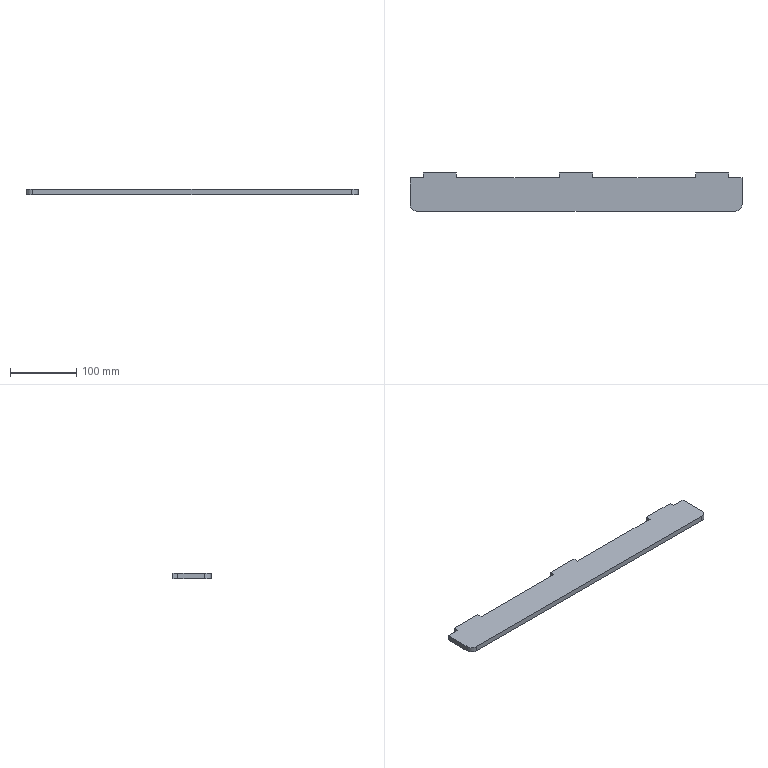Part | SolidWorks | features FlatPattern 1, SMBaseFlange 1, SheetMetal 1 | 1 solid | 20 faces | box 500 x 57.5 x 8 mm | volume 208657 mm3 | plane 18 | cylinder 2 | commonest cylinder face diameters 20 x2
STEP:
#1=CARTESIAN_POINT('',(-172.817,-291.5,0.));
#2=VERTEX_POINT('',#1);
#3=CARTESIAN_POINT('',(-192.817,-291.5,0.));
#4=VERTEX_POINT('',#3);
#5=CARTESIAN_POINT('',(-172.817,-291.5,0.));
#6=DIRECTION('',(-1.,0.,0.));
#7=VECTOR('',#6,1000.);
#8=LINE('',#5,#7);
#9=EDGE_CURVE('',#2,#4,#8,.T.);
#10=ORIENTED_EDGE('',*,*,#9,.F.);
#11=CARTESIAN_POINT('',(-172.817,-291.5,-8.));
#12=VERTEX_POINT('',#11);
#13=CARTESIAN_POINT('',(-172.817,-291.5,-8.));
#14=DIRECTION('',(0.,0.,1.));
#15=VECTOR('',#14,1000.);
#16=LINE('',#13,#15);
#17=EDGE_CURVE('',#12,#2,#16,.T.);
#18=ORIENTED_EDGE('',*,*,#17,.F.);
#19=CARTESIAN_POINT('',(-192.817,-291.5,-8.));
#20=VERTEX_POINT('',#19);
#21=CARTESIAN_POINT('',(-172.817,-291.5,-8.));
#22=DIRECTION('',(-1.,0.,0.));
#23=VECTOR('',#22,1000.);
#24=LINE('',#21,#23);
#25=EDGE_CURVE('',#12,#20,#24,.T.);
#26=ORIENTED_EDGE('',*,*,#25,.T.);
#27=CARTESIAN_POINT('',(-192.817,-291.5,-8.));
#28=DIRECTION('',(0.,0.,1.));
#29=VECTOR('',#28,1000.);
#30=LINE('',#27,#29);
#31=EDGE_CURVE('',#20,#4,#30,.T.);
#32=ORIENTED_EDGE('',*,*,#31,.T.);
#33=EDGE_LOOP('',(#10,#18,#26,#32));
#34=FACE_OUTER_BOUND('',#33,.T.);
#35=CARTESIAN_POINT('',(-172.817,-291.5,-8.));
#36=DIRECTION('',(0.,1.,0.));
#37=DIRECTION('',(0.,0.,1.));
#38=AXIS2_PLACEMENT_3D('',#35,#36,#37);
#39=PLANE('',#38);
#40=ADVANCED_FACE('',(#34),#39,.T.);
#41=CARTESIAN_POINT('',(-172.817,-284.,0.));
#42=VERTEX_POINT('',#41);
#43=CARTESIAN_POINT('',(-172.817,-284.,0.));
#44=DIRECTION('',(0.,-1.,0.));
#45=VECTOR('',#44,1000.);
#46=LINE('',#43,#45);
#47=EDGE_CURVE('',#42,#2,#46,.T.);
#48=ORIENTED_EDGE('',*,*,#47,.F.);
#49=CARTESIAN_POINT('',(-172.817,-284.,-8.));
#50=VERTEX_POINT('',#49);
#51=CARTESIAN_POINT('',(-172.817,-284.,-8.));
#52=DIRECTION('',(0.,0.,1.));
#53=VECTOR('',#52,1000.);
#54=LINE('',#51,#53);
#55=EDGE_CURVE('',#50,#42,#54,.T.);
#56=ORIENTED_EDGE('',*,*,#55,.F.);
#57=CARTESIAN_POINT('',(-172.817,-284.,-8.));
#58=DIRECTION('',(0.,-1.,0.));
#59=VECTOR('',#58,1000.);
#60=LINE('',#57,#59);
#61=EDGE_CURVE('',#50,#12,#60,.T.);
#62=ORIENTED_EDGE('',*,*,#61,.T.);
#63=ORIENTED_EDGE('',*,*,#17,.T.);
#64=EDGE_LOOP('',(#48,#56,#62,#63));
#65=FACE_OUTER_BOUND('',#64,.T.);
#66=CARTESIAN_POINT('',(-172.817,-284.,-8.));
#67=DIRECTION('',(-1.,0.,0.));
#68=DIRECTION('',(0.,-1.,0.));
#69=AXIS2_PLACEMENT_3D('',#66,#67,#68);
#70=PLANE('',#69);
#71=ADVANCED_FACE('',(#65),#70,.T.);
#72=CARTESIAN_POINT('',(-122.817,-284.,0.));
#73=VERTEX_POINT('',#72);
#74=CARTESIAN_POINT('',(-122.817,-284.,0.));
#75=DIRECTION('',(-1.,0.,0.));
#76=VECTOR('',#75,1000.);
#77=LINE('',#74,#76);
#78=EDGE_CURVE('',#73,#42,#77,.T.);
#79=ORIENTED_EDGE('',*,*,#78,.F.);
#80=CARTESIAN_POINT('',(-122.817,-284.,-8.));
#81=VERTEX_POINT('',#80);
#82=CARTESIAN_POINT('',(-122.817,-284.,-8.));
#83=DIRECTION('',(0.,0.,1.));
#84=VECTOR('',#83,1000.);
#85=LINE('',#82,#84);
#86=EDGE_CURVE('',#81,#73,#85,.T.);
#87=ORIENTED_EDGE('',*,*,#86,.F.);
#88=CARTESIAN_POINT('',(-122.817,-284.,-8.));
#89=DIRECTION('',(-1.,0.,0.));
#90=VECTOR('',#89,1000.);
#91=LINE('',#88,#90);
#92=EDGE_CURVE('',#81,#50,#91,.T.);
#93=ORIENTED_EDGE('',*,*,#92,.T.);
#94=ORIENTED_EDGE('',*,*,#55,.T.);
#95=EDGE_LOOP('',(#79,#87,#93,#94));
#96=FACE_OUTER_BOUND('',#95,.T.);
#97=CARTESIAN_POINT('',(-122.817,-284.,-8.));
#98=DIRECTION('',(0.,1.,0.));
#99=DIRECTION('',(0.,0.,1.));
#100=AXIS2_PLACEMENT_3D('',#97,#98,#99);
#101=PLANE('',#100);
#102=ADVANCED_FACE('',(#96),#101,.T.);
#103=CARTESIAN_POINT('',(-122.817,-291.5,0.));
#104=VERTEX_POINT('',#103);
#105=CARTESIAN_POINT('',(-122.817,-291.5,0.));
#106=DIRECTION('',(0.,1.,0.));
#107=VECTOR('',#106,1000.);
#108=LINE('',#105,#107);
#109=EDGE_CURVE('',#104,#73,#108,.T.);
#110=ORIENTED_EDGE('',*,*,#109,.F.);
#111=CARTESIAN_POINT('',(-122.817,-291.5,-8.));
#112=VERTEX_POINT('',#111);
#113=CARTESIAN_POINT('',(-122.817,-291.5,-8.));
#114=DIRECTION('',(0.,0.,1.));
#115=VECTOR('',#114,1000.);
#116=LINE('',#113,#115);
#117=EDGE_CURVE('',#112,#104,#116,.T.);
#118=ORIENTED_EDGE('',*,*,#117,.F.);
#119=CARTESIAN_POINT('',(-122.817,-291.5,-8.));
#120=DIRECTION('',(0.,1.,0.));
#121=VECTOR('',#120,1000.);
#122=LINE('',#119,#121);
#123=EDGE_CURVE('',#112,#81,#122,.T.);
#124=ORIENTED_EDGE('',*,*,#123,.T.);
#125=ORIENTED_EDGE('',*,*,#86,.T.);
#126=EDGE_LOOP('',(#110,#118,#124,#125));
#127=FACE_OUTER_BOUND('',#126,.T.);
#128=CARTESIAN_POINT('',(-122.817,-291.5,-8.));
#129=DIRECTION('',(1.,0.,0.));
#130=DIRECTION('',(0.,0.,-1.));
#131=AXIS2_PLACEMENT_3D('',#128,#129,#130);
#132=PLANE('',#131);
#133=ADVANCED_FACE('',(#127),#132,.T.);
#134=CARTESIAN_POINT('',(32.183,-291.5,0.));
#135=VERTEX_POINT('',#134);
#136=CARTESIAN_POINT('',(32.183,-291.5,0.));
#137=DIRECTION('',(-1.,0.,0.));
#138=VECTOR('',#137,1000.);
#139=LINE('',#136,#138);
#140=EDGE_CURVE('',#135,#104,#139,.T.);
#141=ORIENTED_EDGE('',*,*,#140,.F.);
#142=CARTESIAN_POINT('',(32.183,-291.5,-8.));
#143=VERTEX_POINT('',#142);
#144=CARTESIAN_POINT('',(32.183,-291.5,-8.));
#145=DIRECTION('',(0.,0.,1.));
#146=VECTOR('',#145,1000.);
#147=LINE('',#144,#146);
#148=EDGE_CURVE('',#143,#135,#147,.T.);
#149=ORIENTED_EDGE('',*,*,#148,.F.);
#150=CARTESIAN_POINT('',(32.183,-291.5,-8.));
#151=DIRECTION('',(-1.,0.,0.));
#152=VECTOR('',#151,1000.);
#153=LINE('',#150,#152);
#154=EDGE_CURVE('',#143,#112,#153,.T.);
#155=ORIENTED_EDGE('',*,*,#154,.T.);
#156=ORIENTED_EDGE('',*,*,#117,.T.);
#157=EDGE_LOOP('',(#141,#149,#155,#156));
#158=FACE_OUTER_BOUND('',#157,.T.);
#159=CARTESIAN_POINT('',(32.183,-291.5,-8.));
#160=DIRECTION('',(0.,1.,0.));
#161=DIRECTION('',(0.,0.,1.));
#162=AXIS2_PLACEMENT_3D('',#159,#160,#161);
#163=PLANE('',#162);
#164=ADVANCED_FACE('',(#158),#163,.T.);
#165=CARTESIAN_POINT('',(32.183,-284.,0.));
#166=VERTEX_POINT('',#165);
#167=CARTESIAN_POINT('',(32.183,-284.,0.));
#168=DIRECTION('',(0.,-1.,0.));
#169=VECTOR('',#168,1000.);
#170=LINE('',#167,#169);
#171=EDGE_CURVE('',#166,#135,#170,.T.);
#172=ORIENTED_EDGE('',*,*,#171,.F.);
#173=CARTESIAN_POINT('',(32.183,-284.,-8.));
#174=VERTEX_POINT('',#173);
#175=CARTESIAN_POINT('',(32.183,-284.,-8.));
#176=DIRECTION('',(0.,0.,1.));
#177=VECTOR('',#176,1000.);
#178=LINE('',#175,#177);
#179=EDGE_CURVE('',#174,#166,#178,.T.);
#180=ORIENTED_EDGE('',*,*,#179,.F.);
#181=CARTESIAN_POINT('',(32.183,-284.,-8.));
#182=DIRECTION('',(0.,-1.,0.));
#183=VECTOR('',#182,1000.);
#184=LINE('',#181,#183);
#185=EDGE_CURVE('',#174,#143,#184,.T.);
#186=ORIENTED_EDGE('',*,*,#185,.T.);
#187=ORIENTED_EDGE('',*,*,#148,.T.);
#188=EDGE_LOOP('',(#172,#180,#186,#187));
#189=FACE_OUTER_BOUND('',#188,.T.);
#190=CARTESIAN_POINT('',(32.183,-284.,-8.));
#191=DIRECTION('',(-1.,0.,0.));
#192=DIRECTION('',(0.,-1.,0.));
#193=AXIS2_PLACEMENT_3D('',#190,#191,#192);
#194=PLANE('',#193);
#195=ADVANCED_FACE('',(#189),#194,.T.);
#196=CARTESIAN_POINT('',(82.183,-284.,0.));
#197=VERTEX_POINT('',#196);
#198=CARTESIAN_POINT('',(82.183,-284.,0.));
#199=DIRECTION('',(-1.,0.,0.));
#200=VECTOR('',#199,1000.);
#201=LINE('',#198,#200);
#202=EDGE_CURVE('',#197,#166,#201,.T.);
#203=ORIENTED_EDGE('',*,*,#202,.F.);
#204=CARTESIAN_POINT('',(82.183,-284.,-8.));
#205=VERTEX_POINT('',#204);
#206=CARTESIAN_POINT('',(82.183,-284.,-8.));
#207=DIRECTION('',(0.,0.,1.));
#208=VECTOR('',#207,1000.);
#209=LINE('',#206,#208);
#210=EDGE_CURVE('',#205,#197,#209,.T.);
#211=ORIENTED_EDGE('',*,*,#210,.F.);
#212=CARTESIAN_POINT('',(82.183,-284.,-8.));
#213=DIRECTION('',(-1.,0.,0.));
#214=VECTOR('',#213,1000.);
#215=LINE('',#212,#214);
#216=EDGE_CURVE('',#205,#174,#215,.T.);
#217=ORIENTED_EDGE('',*,*,#216,.T.);
#218=ORIENTED_EDGE('',*,*,#179,.T.);
#219=EDGE_LOOP('',(#203,#211,#217,#218));
#220=FACE_OUTER_BOUND('',#219,.T.);
#221=CARTESIAN_POINT('',(82.183,-284.,-8.));
#222=DIRECTION('',(0.,1.,0.));
#223=DIRECTION('',(0.,0.,1.));
#224=AXIS2_PLACEMENT_3D('',#221,#222,#223);
#225=PLANE('',#224);
#226=ADVANCED_FACE('',(#220),#225,.T.);
#227=CARTESIAN_POINT('',(82.183,-291.5,0.));
#228=VERTEX_POINT('',#227);
#229=CARTESIAN_POINT('',(82.183,-291.5,0.));
#230=DIRECTION('',(0.,1.,0.));
#231=VECTOR('',#230,1000.);
#232=LINE('',#229,#231);
#233=EDGE_CURVE('',#228,#197,#232,.T.);
#234=ORIENTED_EDGE('',*,*,#233,.F.);
#235=CARTESIAN_POINT('',(82.183,-291.5,-8.));
#236=VERTEX_POINT('',#235);
#237=CARTESIAN_POINT('',(82.183,-291.5,-8.));
#238=DIRECTION('',(0.,0.,1.));
#239=VECTOR('',#238,1000.);
#240=LINE('',#237,#239);
#241=EDGE_CURVE('',#236,#228,#240,.T.);
#242=ORIENTED_EDGE('',*,*,#241,.F.);
#243=CARTESIAN_POINT('',(82.183,-291.5,-8.));
#244=DIRECTION('',(0.,1.,0.));
#245=VECTOR('',#244,1000.);
#246=LINE('',#243,#245);
#247=EDGE_CURVE('',#236,#205,#246,.T.);
#248=ORIENTED_EDGE('',*,*,#247,.T.);
#249=ORIENTED_EDGE('',*,*,#210,.T.);
#250=EDGE_LOOP('',(#234,#242,#248,#249));
#251=FACE_OUTER_BOUND('',#250,.T.);
#252=CARTESIAN_POINT('',(82.183,-291.5,-8.));
#253=DIRECTION('',(1.,0.,0.));
#254=DIRECTION('',(0.,1.,0.));
#255=AXIS2_PLACEMENT_3D('',#252,#253,#254);
#256=PLANE('',#255);
#257=ADVANCED_FACE('',(#251),#256,.T.);
#258=CARTESIAN_POINT('',(237.183,-291.5,0.));
#259=VERTEX_POINT('',#258);
#260=CARTESIAN_POINT('',(237.183,-291.5,0.));
#261=DIRECTION('',(-1.,0.,0.));
#262=VECTOR('',#261,1000.);
#263=LINE('',#260,#262);
#264=EDGE_CURVE('',#259,#228,#263,.T.);
#265=ORIENTED_EDGE('',*,*,#264,.F.);
#266=CARTESIAN_POINT('',(237.183,-291.5,-8.));
#267=VERTEX_POINT('',#266);
#268=CARTESIAN_POINT('',(237.183,-291.5,-8.));
#269=DIRECTION('',(0.,0.,1.));
#270=VECTOR('',#269,1000.);
#271=LINE('',#268,#270);
#272=EDGE_CURVE('',#267,#259,#271,.T.);
#273=ORIENTED_EDGE('',*,*,#272,.F.);
#274=CARTESIAN_POINT('',(237.183,-291.5,-8.));
#275=DIRECTION('',(-1.,0.,0.));
#276=VECTOR('',#275,1000.);
#277=LINE('',#274,#276);
#278=EDGE_CURVE('',#267,#236,#277,.T.);
#279=ORIENTED_EDGE('',*,*,#278,.T.);
#280=ORIENTED_EDGE('',*,*,#241,.T.);
#281=EDGE_LOOP('',(#265,#273,#279,#280));
#282=FACE_OUTER_BOUND('',#281,.T.);
#283=CARTESIAN_POINT('',(237.183,-291.5,-8.));
#284=DIRECTION('',(0.,1.,0.));
#285=DIRECTION('',(0.,0.,1.));
#286=AXIS2_PLACEMENT_3D('',#283,#284,#285);
#287=PLANE('',#286);
#288=ADVANCED_FACE('',(#282),#287,.T.);
#289=CARTESIAN_POINT('',(237.183,-284.,0.));
#290=VERTEX_POINT('',#289);
#291=CARTESIAN_POINT('',(237.183,-284.,0.));
#292=DIRECTION('',(0.,-1.,0.));
#293=VECTOR('',#292,1000.);
#294=LINE('',#291,#293);
#295=EDGE_CURVE('',#290,#259,#294,.T.);
#296=ORIENTED_EDGE('',*,*,#295,.F.);
#297=CARTESIAN_POINT('',(237.183,-284.,-8.));
#298=VERTEX_POINT('',#297);
#299=CARTESIAN_POINT('',(237.183,-284.,-8.));
#300=DIRECTION('',(0.,0.,1.));
#301=VECTOR('',#300,1000.);
#302=LINE('',#299,#301);
#303=EDGE_CURVE('',#298,#290,#302,.T.);
#304=ORIENTED_EDGE('',*,*,#303,.F.);
#305=CARTESIAN_POINT('',(237.183,-284.,-8.));
#306=DIRECTION('',(0.,-1.,0.));
#307=VECTOR('',#306,1000.);
#308=LINE('',#305,#307);
#309=EDGE_CURVE('',#298,#267,#308,.T.);
#310=ORIENTED_EDGE('',*,*,#309,.T.);
#311=ORIENTED_EDGE('',*,*,#272,.T.);
#312=EDGE_LOOP('',(#296,#304,#310,#311));
#313=FACE_OUTER_BOUND('',#312,.T.);
#314=CARTESIAN_POINT('',(237.183,-284.,-8.));
#315=DIRECTION('',(-1.,0.,0.));
#316=DIRECTION('',(0.,-1.,0.));
#317=AXIS2_PLACEMENT_3D('',#314,#315,#316);
#318=PLANE('',#317);
#319=ADVANCED_FACE('',(#313),#318,.T.);
#320=CARTESIAN_POINT('',(287.183,-284.,0.));
#321=VERTEX_POINT('',#320);
#322=CARTESIAN_POINT('',(287.183,-284.,0.));
#323=DIRECTION('',(-1.,0.,0.));
#324=VECTOR('',#323,1000.);
#325=LINE('',#322,#324);
#326=EDGE_CURVE('',#321,#290,#325,.T.);
#327=ORIENTED_EDGE('',*,*,#326,.F.);
#328=CARTESIAN_POINT('',(287.183,-284.,-8.));
#329=VERTEX_POINT('',#328);
#330=CARTESIAN_POINT('',(287.183,-284.,-8.));
#331=DIRECTION('',(0.,0.,1.));
#332=VECTOR('',#331,1000.);
#333=LINE('',#330,#332);
#334=EDGE_CURVE('',#329,#321,#333,.T.);
#335=ORIENTED_EDGE('',*,*,#334,.F.);
#336=CARTESIAN_POINT('',(287.183,-284.,-8.));
#337=DIRECTION('',(-1.,0.,0.));
#338=VECTOR('',#337,1000.);
#339=LINE('',#336,#338);
#340=EDGE_CURVE('',#329,#298,#339,.T.);
#341=ORIENTED_EDGE('',*,*,#340,.T.);
#342=ORIENTED_EDGE('',*,*,#303,.T.);
#343=EDGE_LOOP('',(#327,#335,#341,#342));
#344=FACE_OUTER_BOUND('',#343,.T.);
#345=CARTESIAN_POINT('',(287.183,-284.,-8.));
#346=DIRECTION('',(0.,1.,0.));
#347=DIRECTION('',(0.,0.,1.));
#348=AXIS2_PLACEMENT_3D('',#345,#346,#347);
#349=PLANE('',#348);
#350=ADVANCED_FACE('',(#344),#349,.T.);
#351=CARTESIAN_POINT('',(287.183,-291.5,0.));
#352=VERTEX_POINT('',#351);
#353=CARTESIAN_POINT('',(287.183,-291.5,0.));
#354=DIRECTION('',(0.,1.,0.));
#355=VECTOR('',#354,1000.);
#356=LINE('',#353,#355);
#357=EDGE_CURVE('',#352,#321,#356,.T.);
#358=ORIENTED_EDGE('',*,*,#357,.F.);
#359=CARTESIAN_POINT('',(287.183,-291.5,-8.));
#360=VERTEX_POINT('',#359);
#361=CARTESIAN_POINT('',(287.183,-291.5,-8.));
#362=DIRECTION('',(0.,0.,1.));
#363=VECTOR('',#362,1000.);
#364=LINE('',#361,#363);
#365=EDGE_CURVE('',#360,#352,#364,.T.);
#366=ORIENTED_EDGE('',*,*,#365,.F.);
#367=CARTESIAN_POINT('',(287.183,-291.5,-8.));
#368=DIRECTION('',(0.,1.,0.));
#369=VECTOR('',#368,1000.);
#370=LINE('',#367,#369);
#371=EDGE_CURVE('',#360,#329,#370,.T.);
#372=ORIENTED_EDGE('',*,*,#371,.T.);
#373=ORIENTED_EDGE('',*,*,#334,.T.);
#374=EDGE_LOOP('',(#358,#366,#372,#373));
#375=FACE_OUTER_BOUND('',#374,.T.);
#376=CARTESIAN_POINT('',(287.183,-291.5,-8.));
#377=DIRECTION('',(1.,0.,0.));
#378=DIRECTION('',(0.,0.,-1.));
#379=AXIS2_PLACEMENT_3D('',#376,#377,#378);
#380=PLANE('',#379);
#381=ADVANCED_FACE('',(#375),#380,.T.);
#382=CARTESIAN_POINT('',(307.183,-291.5,0.));
#383=VERTEX_POINT('',#382);
#384=CARTESIAN_POINT('',(307.183,-291.5,0.));
#385=DIRECTION('',(-1.,0.,0.));
#386=VECTOR('',#385,1000.);
#387=LINE('',#384,#386);
#388=EDGE_CURVE('',#383,#352,#387,.T.);
#389=ORIENTED_EDGE('',*,*,#388,.F.);
#390=CARTESIAN_POINT('',(307.183,-291.5,-8.));
#391=VERTEX_POINT('',#390);
#392=CARTESIAN_POINT('',(307.183,-291.5,-8.));
#393=DIRECTION('',(0.,0.,1.));
#394=VECTOR('',#393,1000.);
#395=LINE('',#392,#394);
#396=EDGE_CURVE('',#391,#383,#395,.T.);
#397=ORIENTED_EDGE('',*,*,#396,.F.);
#398=CARTESIAN_POINT('',(307.183,-291.5,-8.));
#399=DIRECTION('',(-1.,0.,0.));
#400=VECTOR('',#399,1000.);
#401=LINE('',#398,#400);
#402=EDGE_CURVE('',#391,#360,#401,.T.);
#403=ORIENTED_EDGE('',*,*,#402,.T.);
#404=ORIENTED_EDGE('',*,*,#365,.T.);
#405=EDGE_LOOP('',(#389,#397,#403,#404));
#406=FACE_OUTER_BOUND('',#405,.T.);
#407=CARTESIAN_POINT('',(307.183,-291.5,-8.));
#408=DIRECTION('',(0.,1.,0.));
#409=DIRECTION('',(0.,0.,1.));
#410=AXIS2_PLACEMENT_3D('',#407,#408,#409);
#411=PLANE('',#410);
#412=ADVANCED_FACE('',(#406),#411,.T.);
#413=CARTESIAN_POINT('',(307.183,-331.5,0.));
#414=VERTEX_POINT('',#413);
#415=CARTESIAN_POINT('',(307.183,-331.5,0.));
#416=DIRECTION('',(0.,1.,0.));
#417=VECTOR('',#416,1000.);
#418=LINE('',#415,#417);
#419=EDGE_CURVE('',#414,#383,#418,.T.);
#420=ORIENTED_EDGE('',*,*,#419,.F.);
#421=CARTESIAN_POINT('',(307.183,-331.5,-8.));
#422=VERTEX_POINT('',#421);
#423=CARTESIAN_POINT('',(307.183,-331.5,-8.));
#424=DIRECTION('',(0.,0.,1.));
#425=VECTOR('',#424,1000.);
#426=LINE('',#423,#425);
#427=EDGE_CURVE('',#422,#414,#426,.T.);
#428=ORIENTED_EDGE('',*,*,#427,.F.);
#429=CARTESIAN_POINT('',(307.183,-331.5,-8.));
#430=DIRECTION('',(0.,1.,0.));
#431=VECTOR('',#430,1000.);
#432=LINE('',#429,#431);
#433=EDGE_CURVE('',#422,#391,#432,.T.);
#434=ORIENTED_EDGE('',*,*,#433,.T.);
#435=ORIENTED_EDGE('',*,*,#396,.T.);
#436=EDGE_LOOP('',(#420,#428,#434,#435));
#437=FACE_OUTER_BOUND('',#436,.T.);
#438=CARTESIAN_POINT('',(307.183,-331.5,-8.));
#439=DIRECTION('',(1.,0.,0.));
#440=DIRECTION('',(0.,1.,0.));
#441=AXIS2_PLACEMENT_3D('',#438,#439,#440);
#442=PLANE('',#441);
#443=ADVANCED_FACE('',(#437),#442,.T.);
#444=CARTESIAN_POINT('',(297.183,-341.5,0.));
#445=VERTEX_POINT('',#444);
#446=CARTESIAN_POINT('',(297.183,-331.5,0.));
#447=DIRECTION('',(0.,0.,1.));
#448=DIRECTION('',(1.,0.,0.));
#449=AXIS2_PLACEMENT_3D('',#446,#447,#448);
#450=CIRCLE('',#449,10.);
#451=EDGE_CURVE('',#445,#414,#450,.T.);
#452=ORIENTED_EDGE('',*,*,#451,.F.);
#453=CARTESIAN_POINT('',(297.183,-341.5,-8.));
#454=VERTEX_POINT('',#453);
#455=CARTESIAN_POINT('',(297.183,-341.5,-8.));
#456=DIRECTION('',(0.,0.,1.));
#457=VECTOR('',#456,1000.);
#458=LINE('',#455,#457);
#459=EDGE_CURVE('',#454,#445,#458,.T.);
#460=ORIENTED_EDGE('',*,*,#459,.F.);
#461=CARTESIAN_POINT('',(297.183,-331.5,-8.));
#462=DIRECTION('',(0.,0.,1.));
#463=DIRECTION('',(1.,0.,0.));
#464=AXIS2_PLACEMENT_3D('',#461,#462,#463);
#465=CIRCLE('',#464,10.);
#466=EDGE_CURVE('',#454,#422,#465,.T.);
#467=ORIENTED_EDGE('',*,*,#466,.T.);
#468=ORIENTED_EDGE('',*,*,#427,.T.);
#469=EDGE_LOOP('',(#452,#460,#467,#468));
#470=FACE_OUTER_BOUND('',#469,.T.);
#471=CARTESIAN_POINT('',(297.183,-331.5,-8.));
#472=DIRECTION('',(0.,0.,1.));
#473=DIRECTION('',(1.,0.,0.));
#474=AXIS2_PLACEMENT_3D('',#471,#472,#473);
#475=CYLINDRICAL_SURFACE('',#474,10.);
#476=ADVANCED_FACE('',(#470),#475,.T.);
#477=CARTESIAN_POINT('',(-182.817,-341.5,0.));
#478=VERTEX_POINT('',#477);
#479=CARTESIAN_POINT('',(-182.817,-341.5,0.));
#480=DIRECTION('',(1.,0.,0.));
#481=VECTOR('',#480,1000.);
#482=LINE('',#479,#481);
#483=EDGE_CURVE('',#478,#445,#482,.T.);
#484=ORIENTED_EDGE('',*,*,#483,.F.);
#485=CARTESIAN_POINT('',(-182.817,-341.5,-8.));
#486=VERTEX_POINT('',#485);
#487=CARTESIAN_POINT('',(-182.817,-341.5,-8.));
#488=DIRECTION('',(0.,0.,1.));
#489=VECTOR('',#488,1000.);
#490=LINE('',#487,#489);
#491=EDGE_CURVE('',#486,#478,#490,.T.);
#492=ORIENTED_EDGE('',*,*,#491,.F.);
#493=CARTESIAN_POINT('',(-182.817,-341.5,-8.));
#494=DIRECTION('',(1.,0.,0.));
#495=VECTOR('',#494,1000.);
#496=LINE('',#493,#495);
#497=EDGE_CURVE('',#486,#454,#496,.T.);
#498=ORIENTED_EDGE('',*,*,#497,.T.);
#499=ORIENTED_EDGE('',*,*,#459,.T.);
#500=EDGE_LOOP('',(#484,#492,#498,#499));
#501=FACE_OUTER_BOUND('',#500,.T.);
#502=CARTESIAN_POINT('',(-182.817,-341.5,-8.));
#503=DIRECTION('',(0.,-1.,0.));
#504=DIRECTION('',(0.,0.,-1.));
#505=AXIS2_PLACEMENT_3D('',#502,#503,#504);
#506=PLANE('',#505);
#507=ADVANCED_FACE('',(#501),#506,.T.);
#508=CARTESIAN_POINT('',(-192.817,-331.5,0.));
#509=VERTEX_POINT('',#508);
#510=CARTESIAN_POINT('',(-182.817,-331.5,0.));
#511=DIRECTION('',(0.,0.,1.));
#512=DIRECTION('',(1.,0.,0.));
#513=AXIS2_PLACEMENT_3D('',#510,#511,#512);
#514=CIRCLE('',#513,10.);
#515=EDGE_CURVE('',#509,#478,#514,.T.);
#516=ORIENTED_EDGE('',*,*,#515,.F.);
#517=CARTESIAN_POINT('',(-192.817,-331.5,-8.));
#518=VERTEX_POINT('',#517);
#519=CARTESIAN_POINT('',(-192.817,-331.5,-8.));
#520=DIRECTION('',(0.,0.,1.));
#521=VECTOR('',#520,1000.);
#522=LINE('',#519,#521);
#523=EDGE_CURVE('',#518,#509,#522,.T.);
#524=ORIENTED_EDGE('',*,*,#523,.F.);
#525=CARTESIAN_POINT('',(-182.817,-331.5,-8.));
#526=DIRECTION('',(0.,0.,1.));
#527=DIRECTION('',(1.,0.,0.));
#528=AXIS2_PLACEMENT_3D('',#525,#526,#527);
#529=CIRCLE('',#528,10.);
#530=EDGE_CURVE('',#518,#486,#529,.T.);
#531=ORIENTED_EDGE('',*,*,#530,.T.);
#532=ORIENTED_EDGE('',*,*,#491,.T.);
#533=EDGE_LOOP('',(#516,#524,#531,#532));
#534=FACE_OUTER_BOUND('',#533,.T.);
#535=CARTESIAN_POINT('',(-182.817,-331.5,-8.));
#536=DIRECTION('',(0.,0.,1.));
#537=DIRECTION('',(1.,0.,0.));
#538=AXIS2_PLACEMENT_3D('',#535,#536,#537);
#539=CYLINDRICAL_SURFACE('',#538,10.);
#540=ADVANCED_FACE('',(#534),#539,.T.);
#541=CARTESIAN_POINT('',(-192.817,-291.5,0.));
#542=DIRECTION('',(0.,-1.,0.));
#543=VECTOR('',#542,1000.);
#544=LINE('',#541,#543);
#545=EDGE_CURVE('',#4,#509,#544,.T.);
#546=ORIENTED_EDGE('',*,*,#545,.F.);
#547=ORIENTED_EDGE('',*,*,#31,.F.);
#548=CARTESIAN_POINT('',(-192.817,-291.5,-8.));
#549=DIRECTION('',(0.,-1.,0.));
#550=VECTOR('',#549,1000.);
#551=LINE('',#548,#550);
#552=EDGE_CURVE('',#20,#518,#551,.T.);
#553=ORIENTED_EDGE('',*,*,#552,.T.);
#554=ORIENTED_EDGE('',*,*,#523,.T.);
#555=EDGE_LOOP('',(#546,#547,#553,#554));
#556=FACE_OUTER_BOUND('',#555,.T.);
#557=CARTESIAN_POINT('',(-192.817,-291.5,-8.));
#558=DIRECTION('',(-1.,0.,0.));
#559=DIRECTION('',(0.,0.,1.));
#560=AXIS2_PLACEMENT_3D('',#557,#558,#559);
#561=PLANE('',#560);
#562=ADVANCED_FACE('',(#556),#561,.T.);
#563=ORIENTED_EDGE('',*,*,#25,.F.);
#564=ORIENTED_EDGE('',*,*,#61,.F.);
#565=ORIENTED_EDGE('',*,*,#92,.F.);
#566=ORIENTED_EDGE('',*,*,#123,.F.);
#567=ORIENTED_EDGE('',*,*,#154,.F.);
#568=ORIENTED_EDGE('',*,*,#185,.F.);
#569=ORIENTED_EDGE('',*,*,#216,.F.);
#570=ORIENTED_EDGE('',*,*,#247,.F.);
#571=ORIENTED_EDGE('',*,*,#278,.F.);
#572=ORIENTED_EDGE('',*,*,#309,.F.);
#573=ORIENTED_EDGE('',*,*,#340,.F.);
#574=ORIENTED_EDGE('',*,*,#371,.F.);
#575=ORIENTED_EDGE('',*,*,#402,.F.);
#576=ORIENTED_EDGE('',*,*,#433,.F.);
#577=ORIENTED_EDGE('',*,*,#466,.F.);
#578=ORIENTED_EDGE('',*,*,#497,.F.);
#579=ORIENTED_EDGE('',*,*,#530,.F.);
#580=ORIENTED_EDGE('',*,*,#552,.F.);
#581=EDGE_LOOP('',(#563,#564,#565,#566,#567,#568,#569,#570,#571,#572,#573,#574,#575,#576,#577,#578,#579,#580));
#582=FACE_OUTER_BOUND('',#581,.T.);
#583=CARTESIAN_POINT('',(-182.817,-331.5,-8.));
#584=DIRECTION('',(0.,0.,1.));
#585=DIRECTION('',(1.,0.,0.));
#586=AXIS2_PLACEMENT_3D('',#583,#584,#585);
#587=PLANE('',#586);
#588=ADVANCED_FACE('',(#582),#587,.F.);
#589=ORIENTED_EDGE('',*,*,#9,.T.);
#590=ORIENTED_EDGE('',*,*,#545,.T.);
#591=ORIENTED_EDGE('',*,*,#515,.T.);
#592=ORIENTED_EDGE('',*,*,#483,.T.);
#593=ORIENTED_EDGE('',*,*,#451,.T.);
#594=ORIENTED_EDGE('',*,*,#419,.T.);
#595=ORIENTED_EDGE('',*,*,#388,.T.);
#596=ORIENTED_EDGE('',*,*,#357,.T.);
#597=ORIENTED_EDGE('',*,*,#326,.T.);
#598=ORIENTED_EDGE('',*,*,#295,.T.);
#599=ORIENTED_EDGE('',*,*,#264,.T.);
#600=ORIENTED_EDGE('',*,*,#233,.T.);
#601=ORIENTED_EDGE('',*,*,#202,.T.);
#602=ORIENTED_EDGE('',*,*,#171,.T.);
#603=ORIENTED_EDGE('',*,*,#140,.T.);
#604=ORIENTED_EDGE('',*,*,#109,.T.);
#605=ORIENTED_EDGE('',*,*,#78,.T.);
#606=ORIENTED_EDGE('',*,*,#47,.T.);
#607=EDGE_LOOP('',(#589,#590,#591,#592,#593,#594,#595,#596,#597,#598,#599,#600,#601,#602,#603,#604,#605,#606));
#608=FACE_OUTER_BOUND('',#607,.T.);
#609=CARTESIAN_POINT('',(-182.817,-331.5,0.));
#610=DIRECTION('',(0.,0.,1.));
#611=DIRECTION('',(1.,0.,0.));
#612=AXIS2_PLACEMENT_3D('',#609,#610,#611);
#613=PLANE('',#612);
#614=ADVANCED_FACE('',(#608),#613,.T.);
#615=CLOSED_SHELL('',(#40,#71,#102,#133,#164,#195,#226,#257,#288,#319,#350,#381,#412,#443,#476,#507,#540,#562,#588,#614));
#616=MANIFOLD_SOLID_BREP('',#615);
#617=CARTESIAN_POINT('',(0.,0.,0.));
#618=DIRECTION('',(0.,0.,1.));
#619=DIRECTION('',(1.,0.,0.));
#620=AXIS2_PLACEMENT_3D('',#617,#618,#619);
#621=(LENGTH_UNIT()NAMED_UNIT(*)SI_UNIT(.MILLI.,.METRE.));
#622=UNCERTAINTY_MEASURE_WITH_UNIT(LENGTH_MEASURE(0.00001),#621,'','');
#623=(NAMED_UNIT(*)PLANE_ANGLE_UNIT()SI_UNIT($,.RADIAN.));
#624=(NAMED_UNIT(*)SI_UNIT($,.STERADIAN.)SOLID_ANGLE_UNIT());
#625=(GEOMETRIC_REPRESENTATION_CONTEXT(3)GLOBAL_UNCERTAINTY_ASSIGNED_CONTEXT((#622))GLOBAL_UNIT_ASSIGNED_CONTEXT((#621,#623,#624))REPRESENTATION_CONTEXT('',''));
#626=ADVANCED_BREP_SHAPE_REPRESENTATION('',(#616,#620),#625);